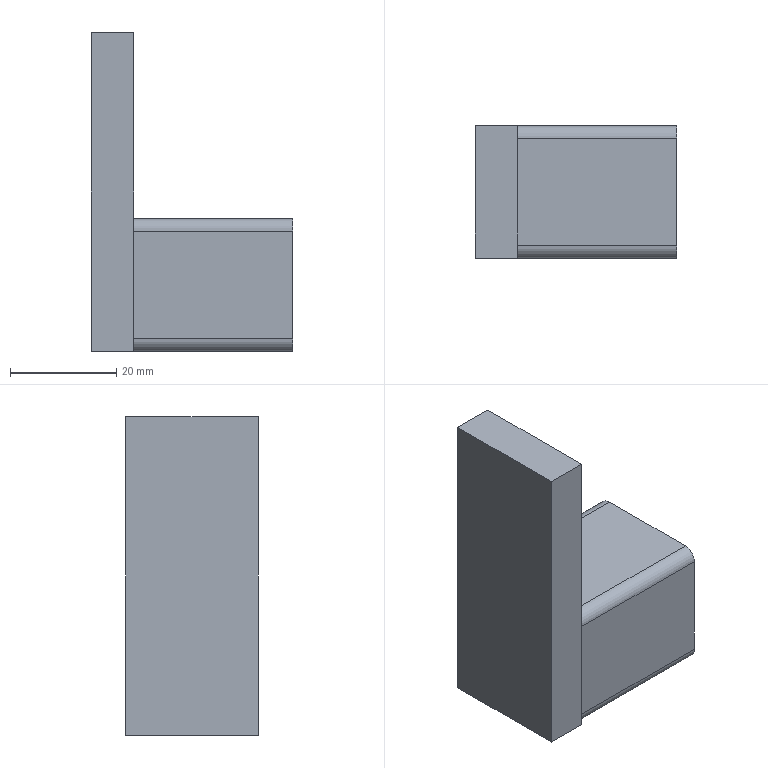Part | SolidWorks | features ICE 1, WeldMemberFeat 1, WeldmentFeature 1 | 2 solids | 24 faces | box 38 x 25 x 60 mm | volume 15316 mm3 | plane 16 | cylinder 8 | commonest cylinder face diameters 2.4 x4 4.8 x4
STEP:
#1=CARTESIAN_POINT('',(-15.,10.1,-12.5));
#2=VERTEX_POINT('',#1);
#3=CARTESIAN_POINT('',(-15.,12.5,-10.1));
#4=VERTEX_POINT('',#3);
#5=CARTESIAN_POINT('',(-15.,10.1,-10.1));
#6=DIRECTION('',(1.,0.,0.));
#7=DIRECTION('',(0.,0.,-1.));
#8=AXIS2_PLACEMENT_3D('',#5,#6,#7);
#9=CIRCLE('',#8,2.4);
#10=EDGE_CURVE('',#2,#4,#9,.T.);
#11=ORIENTED_EDGE('',*,*,#10,.T.);
#12=CARTESIAN_POINT('',(15.,12.5,-10.1));
#13=VERTEX_POINT('',#12);
#14=CARTESIAN_POINT('',(15.,12.5,-10.1));
#15=DIRECTION('',(-1.,0.,0.));
#16=VECTOR('',#15,1000.);
#17=LINE('',#14,#16);
#18=EDGE_CURVE('',#13,#4,#17,.T.);
#19=ORIENTED_EDGE('',*,*,#18,.F.);
#20=CARTESIAN_POINT('',(15.,10.1,-12.5));
#21=VERTEX_POINT('',#20);
#22=CARTESIAN_POINT('',(15.,10.1,-10.1));
#23=DIRECTION('',(1.,0.,0.));
#24=DIRECTION('',(0.,0.,-1.));
#25=AXIS2_PLACEMENT_3D('',#22,#23,#24);
#26=CIRCLE('',#25,2.4);
#27=EDGE_CURVE('',#21,#13,#26,.T.);
#28=ORIENTED_EDGE('',*,*,#27,.F.);
#29=CARTESIAN_POINT('',(15.,10.1,-12.5));
#30=DIRECTION('',(-1.,0.,0.));
#31=VECTOR('',#30,1000.);
#32=LINE('',#29,#31);
#33=EDGE_CURVE('',#21,#2,#32,.T.);
#34=ORIENTED_EDGE('',*,*,#33,.T.);
#35=EDGE_LOOP('',(#11,#19,#28,#34));
#36=FACE_OUTER_BOUND('',#35,.T.);
#37=CARTESIAN_POINT('',(15.,10.1,-10.1));
#38=DIRECTION('',(-1.,0.,0.));
#39=DIRECTION('',(0.,0.,1.));
#40=AXIS2_PLACEMENT_3D('',#37,#38,#39);
#41=CYLINDRICAL_SURFACE('',#40,2.4);
#42=ADVANCED_FACE('',(#36),#41,.T.);
#43=CARTESIAN_POINT('',(-15.,12.5,10.1));
#44=VERTEX_POINT('',#43);
#45=CARTESIAN_POINT('',(-15.,12.5,-10.1));
#46=DIRECTION('',(0.,0.,1.));
#47=VECTOR('',#46,1000.);
#48=LINE('',#45,#47);
#49=EDGE_CURVE('',#4,#44,#48,.T.);
#50=ORIENTED_EDGE('',*,*,#49,.T.);
#51=CARTESIAN_POINT('',(15.,12.5,10.1));
#52=VERTEX_POINT('',#51);
#53=CARTESIAN_POINT('',(15.,12.5,10.1));
#54=DIRECTION('',(-1.,0.,0.));
#55=VECTOR('',#54,1000.);
#56=LINE('',#53,#55);
#57=EDGE_CURVE('',#52,#44,#56,.T.);
#58=ORIENTED_EDGE('',*,*,#57,.F.);
#59=CARTESIAN_POINT('',(15.,12.5,-10.1));
#60=DIRECTION('',(0.,0.,1.));
#61=VECTOR('',#60,1000.);
#62=LINE('',#59,#61);
#63=EDGE_CURVE('',#13,#52,#62,.T.);
#64=ORIENTED_EDGE('',*,*,#63,.F.);
#65=ORIENTED_EDGE('',*,*,#18,.T.);
#66=EDGE_LOOP('',(#50,#58,#64,#65));
#67=FACE_OUTER_BOUND('',#66,.T.);
#68=CARTESIAN_POINT('',(15.,12.5,-10.1));
#69=DIRECTION('',(0.,-1.,0.));
#70=DIRECTION('',(0.,0.,-1.));
#71=AXIS2_PLACEMENT_3D('',#68,#69,#70);
#72=PLANE('',#71);
#73=ADVANCED_FACE('',(#67),#72,.F.);
#74=CARTESIAN_POINT('',(-15.,10.1,12.5));
#75=VERTEX_POINT('',#74);
#76=CARTESIAN_POINT('',(-15.,10.1,10.1));
#77=DIRECTION('',(1.,0.,0.));
#78=DIRECTION('',(0.,0.,-1.));
#79=AXIS2_PLACEMENT_3D('',#76,#77,#78);
#80=CIRCLE('',#79,2.4);
#81=EDGE_CURVE('',#44,#75,#80,.T.);
#82=ORIENTED_EDGE('',*,*,#81,.T.);
#83=CARTESIAN_POINT('',(15.,10.1,12.5));
#84=VERTEX_POINT('',#83);
#85=CARTESIAN_POINT('',(15.,10.1,12.5));
#86=DIRECTION('',(-1.,0.,0.));
#87=VECTOR('',#86,1000.);
#88=LINE('',#85,#87);
#89=EDGE_CURVE('',#84,#75,#88,.T.);
#90=ORIENTED_EDGE('',*,*,#89,.F.);
#91=CARTESIAN_POINT('',(15.,10.1,10.1));
#92=DIRECTION('',(1.,0.,0.));
#93=DIRECTION('',(0.,0.,-1.));
#94=AXIS2_PLACEMENT_3D('',#91,#92,#93);
#95=CIRCLE('',#94,2.4);
#96=EDGE_CURVE('',#52,#84,#95,.T.);
#97=ORIENTED_EDGE('',*,*,#96,.F.);
#98=ORIENTED_EDGE('',*,*,#57,.T.);
#99=EDGE_LOOP('',(#82,#90,#97,#98));
#100=FACE_OUTER_BOUND('',#99,.T.);
#101=CARTESIAN_POINT('',(15.,10.1,10.1));
#102=DIRECTION('',(-1.,0.,0.));
#103=DIRECTION('',(0.,0.,1.));
#104=AXIS2_PLACEMENT_3D('',#101,#102,#103);
#105=CYLINDRICAL_SURFACE('',#104,2.4);
#106=ADVANCED_FACE('',(#100),#105,.T.);
#107=CARTESIAN_POINT('',(-15.,-10.1,12.5));
#108=VERTEX_POINT('',#107);
#109=CARTESIAN_POINT('',(-15.,-10.1,12.5));
#110=DIRECTION('',(0.,-1.,0.));
#111=VECTOR('',#110,1000.);
#112=LINE('',#109,#111);
#113=EDGE_CURVE('',#75,#108,#112,.T.);
#114=ORIENTED_EDGE('',*,*,#113,.T.);
#115=CARTESIAN_POINT('',(15.,-10.1,12.5));
#116=VERTEX_POINT('',#115);
#117=CARTESIAN_POINT('',(15.,-10.1,12.5));
#118=DIRECTION('',(-1.,0.,0.));
#119=VECTOR('',#118,1000.);
#120=LINE('',#117,#119);
#121=EDGE_CURVE('',#116,#108,#120,.T.);
#122=ORIENTED_EDGE('',*,*,#121,.F.);
#123=CARTESIAN_POINT('',(15.,-10.1,12.5));
#124=DIRECTION('',(0.,-1.,0.));
#125=VECTOR('',#124,1000.);
#126=LINE('',#123,#125);
#127=EDGE_CURVE('',#84,#116,#126,.T.);
#128=ORIENTED_EDGE('',*,*,#127,.F.);
#129=ORIENTED_EDGE('',*,*,#89,.T.);
#130=EDGE_LOOP('',(#114,#122,#128,#129));
#131=FACE_OUTER_BOUND('',#130,.T.);
#132=CARTESIAN_POINT('',(15.,-10.1,12.5));
#133=DIRECTION('',(0.,0.,-1.));
#134=DIRECTION('',(-1.,0.,0.));
#135=AXIS2_PLACEMENT_3D('',#132,#133,#134);
#136=PLANE('',#135);
#137=ADVANCED_FACE('',(#131),#136,.F.);
#138=CARTESIAN_POINT('',(-15.,-12.5,10.1));
#139=VERTEX_POINT('',#138);
#140=CARTESIAN_POINT('',(-15.,-10.1,10.1));
#141=DIRECTION('',(1.,0.,0.));
#142=DIRECTION('',(0.,0.,-1.));
#143=AXIS2_PLACEMENT_3D('',#140,#141,#142);
#144=CIRCLE('',#143,2.4);
#145=EDGE_CURVE('',#108,#139,#144,.T.);
#146=ORIENTED_EDGE('',*,*,#145,.T.);
#147=CARTESIAN_POINT('',(15.,-12.5,10.1));
#148=VERTEX_POINT('',#147);
#149=CARTESIAN_POINT('',(15.,-12.5,10.1));
#150=DIRECTION('',(-1.,0.,0.));
#151=VECTOR('',#150,1000.);
#152=LINE('',#149,#151);
#153=EDGE_CURVE('',#148,#139,#152,.T.);
#154=ORIENTED_EDGE('',*,*,#153,.F.);
#155=CARTESIAN_POINT('',(15.,-10.1,10.1));
#156=DIRECTION('',(1.,0.,0.));
#157=DIRECTION('',(0.,0.,-1.));
#158=AXIS2_PLACEMENT_3D('',#155,#156,#157);
#159=CIRCLE('',#158,2.4);
#160=EDGE_CURVE('',#116,#148,#159,.T.);
#161=ORIENTED_EDGE('',*,*,#160,.F.);
#162=ORIENTED_EDGE('',*,*,#121,.T.);
#163=EDGE_LOOP('',(#146,#154,#161,#162));
#164=FACE_OUTER_BOUND('',#163,.T.);
#165=CARTESIAN_POINT('',(15.,-10.1,10.1));
#166=DIRECTION('',(-1.,0.,0.));
#167=DIRECTION('',(0.,0.,1.));
#168=AXIS2_PLACEMENT_3D('',#165,#166,#167);
#169=CYLINDRICAL_SURFACE('',#168,2.4);
#170=ADVANCED_FACE('',(#164),#169,.T.);
#171=CARTESIAN_POINT('',(-15.,-12.5,-10.1));
#172=VERTEX_POINT('',#171);
#173=CARTESIAN_POINT('',(-15.,-12.5,10.1));
#174=DIRECTION('',(0.,0.,-1.));
#175=VECTOR('',#174,1000.);
#176=LINE('',#173,#175);
#177=EDGE_CURVE('',#139,#172,#176,.T.);
#178=ORIENTED_EDGE('',*,*,#177,.T.);
#179=CARTESIAN_POINT('',(15.,-12.5,-10.1));
#180=VERTEX_POINT('',#179);
#181=CARTESIAN_POINT('',(15.,-12.5,-10.1));
#182=DIRECTION('',(-1.,0.,0.));
#183=VECTOR('',#182,1000.);
#184=LINE('',#181,#183);
#185=EDGE_CURVE('',#180,#172,#184,.T.);
#186=ORIENTED_EDGE('',*,*,#185,.F.);
#187=CARTESIAN_POINT('',(15.,-12.5,10.1));
#188=DIRECTION('',(0.,0.,-1.));
#189=VECTOR('',#188,1000.);
#190=LINE('',#187,#189);
#191=EDGE_CURVE('',#148,#180,#190,.T.);
#192=ORIENTED_EDGE('',*,*,#191,.F.);
#193=ORIENTED_EDGE('',*,*,#153,.T.);
#194=EDGE_LOOP('',(#178,#186,#192,#193));
#195=FACE_OUTER_BOUND('',#194,.T.);
#196=CARTESIAN_POINT('',(15.,-12.5,10.1));
#197=DIRECTION('',(0.,1.,0.));
#198=DIRECTION('',(0.,0.,1.));
#199=AXIS2_PLACEMENT_3D('',#196,#197,#198);
#200=PLANE('',#199);
#201=ADVANCED_FACE('',(#195),#200,.F.);
#202=CARTESIAN_POINT('',(-15.,-10.1,-12.5));
#203=VERTEX_POINT('',#202);
#204=CARTESIAN_POINT('',(-15.,-10.1,-10.1));
#205=DIRECTION('',(1.,0.,0.));
#206=DIRECTION('',(0.,0.,-1.));
#207=AXIS2_PLACEMENT_3D('',#204,#205,#206);
#208=CIRCLE('',#207,2.4);
#209=EDGE_CURVE('',#172,#203,#208,.T.);
#210=ORIENTED_EDGE('',*,*,#209,.T.);
#211=CARTESIAN_POINT('',(15.,-10.1,-12.5));
#212=VERTEX_POINT('',#211);
#213=CARTESIAN_POINT('',(15.,-10.1,-12.5));
#214=DIRECTION('',(-1.,0.,0.));
#215=VECTOR('',#214,1000.);
#216=LINE('',#213,#215);
#217=EDGE_CURVE('',#212,#203,#216,.T.);
#218=ORIENTED_EDGE('',*,*,#217,.F.);
#219=CARTESIAN_POINT('',(15.,-10.1,-10.1));
#220=DIRECTION('',(1.,0.,0.));
#221=DIRECTION('',(0.,0.,-1.));
#222=AXIS2_PLACEMENT_3D('',#219,#220,#221);
#223=CIRCLE('',#222,2.4);
#224=EDGE_CURVE('',#180,#212,#223,.T.);
#225=ORIENTED_EDGE('',*,*,#224,.F.);
#226=ORIENTED_EDGE('',*,*,#185,.T.);
#227=EDGE_LOOP('',(#210,#218,#225,#226));
#228=FACE_OUTER_BOUND('',#227,.T.);
#229=CARTESIAN_POINT('',(15.,-10.1,-10.1));
#230=DIRECTION('',(-1.,0.,0.));
#231=DIRECTION('',(0.,0.,1.));
#232=AXIS2_PLACEMENT_3D('',#229,#230,#231);
#233=CYLINDRICAL_SURFACE('',#232,2.4);
#234=ADVANCED_FACE('',(#228),#233,.T.);
#235=CARTESIAN_POINT('',(-15.,11.3,10.1));
#236=VERTEX_POINT('',#235);
#237=CARTESIAN_POINT('',(-15.,10.1,11.3));
#238=VERTEX_POINT('',#237);
#239=CARTESIAN_POINT('',(-15.,10.1,10.1));
#240=DIRECTION('',(1.,0.,0.));
#241=DIRECTION('',(0.,0.,-1.));
#242=AXIS2_PLACEMENT_3D('',#239,#240,#241);
#243=CIRCLE('',#242,1.2);
#244=EDGE_CURVE('',#236,#238,#243,.T.);
#245=ORIENTED_EDGE('',*,*,#244,.F.);
#246=CARTESIAN_POINT('',(15.,11.3,10.1));
#247=VERTEX_POINT('',#246);
#248=CARTESIAN_POINT('',(15.,11.3,10.1));
#249=DIRECTION('',(-1.,0.,0.));
#250=VECTOR('',#249,1000.);
#251=LINE('',#248,#250);
#252=EDGE_CURVE('',#247,#236,#251,.T.);
#253=ORIENTED_EDGE('',*,*,#252,.F.);
#254=CARTESIAN_POINT('',(15.,10.1,11.3));
#255=VERTEX_POINT('',#254);
#256=CARTESIAN_POINT('',(15.,10.1,10.1));
#257=DIRECTION('',(1.,0.,0.));
#258=DIRECTION('',(0.,0.,-1.));
#259=AXIS2_PLACEMENT_3D('',#256,#257,#258);
#260=CIRCLE('',#259,1.2);
#261=EDGE_CURVE('',#247,#255,#260,.T.);
#262=ORIENTED_EDGE('',*,*,#261,.T.);
#263=CARTESIAN_POINT('',(15.,10.1,11.3));
#264=DIRECTION('',(-1.,0.,0.));
#265=VECTOR('',#264,1000.);
#266=LINE('',#263,#265);
#267=EDGE_CURVE('',#255,#238,#266,.T.);
#268=ORIENTED_EDGE('',*,*,#267,.T.);
#269=EDGE_LOOP('',(#245,#253,#262,#268));
#270=FACE_OUTER_BOUND('',#269,.T.);
#271=CARTESIAN_POINT('',(15.,10.1,10.1));
#272=DIRECTION('',(-1.,0.,0.));
#273=DIRECTION('',(0.,0.,1.));
#274=AXIS2_PLACEMENT_3D('',#271,#272,#273);
#275=CYLINDRICAL_SURFACE('',#274,1.2);
#276=ADVANCED_FACE('',(#270),#275,.F.);
#277=CARTESIAN_POINT('',(-15.,11.3,-10.1));
#278=VERTEX_POINT('',#277);
#279=CARTESIAN_POINT('',(-15.,11.3,-10.1));
#280=DIRECTION('',(0.,0.,1.));
#281=VECTOR('',#280,1000.);
#282=LINE('',#279,#281);
#283=EDGE_CURVE('',#278,#236,#282,.T.);
#284=ORIENTED_EDGE('',*,*,#283,.F.);
#285=CARTESIAN_POINT('',(15.,11.3,-10.1));
#286=VERTEX_POINT('',#285);
#287=CARTESIAN_POINT('',(15.,11.3,-10.1));
#288=DIRECTION('',(-1.,0.,0.));
#289=VECTOR('',#288,1000.);
#290=LINE('',#287,#289);
#291=EDGE_CURVE('',#286,#278,#290,.T.);
#292=ORIENTED_EDGE('',*,*,#291,.F.);
#293=CARTESIAN_POINT('',(15.,11.3,-10.1));
#294=DIRECTION('',(0.,0.,1.));
#295=VECTOR('',#294,1000.);
#296=LINE('',#293,#295);
#297=EDGE_CURVE('',#286,#247,#296,.T.);
#298=ORIENTED_EDGE('',*,*,#297,.T.);
#299=ORIENTED_EDGE('',*,*,#252,.T.);
#300=EDGE_LOOP('',(#284,#292,#298,#299));
#301=FACE_OUTER_BOUND('',#300,.T.);
#302=CARTESIAN_POINT('',(15.,11.3,-10.1));
#303=DIRECTION('',(0.,-1.,0.));
#304=DIRECTION('',(0.,0.,-1.));
#305=AXIS2_PLACEMENT_3D('',#302,#303,#304);
#306=PLANE('',#305);
#307=ADVANCED_FACE('',(#301),#306,.T.);
#308=CARTESIAN_POINT('',(-15.,10.1,-11.3));
#309=VERTEX_POINT('',#308);
#310=CARTESIAN_POINT('',(-15.,10.1,-10.1));
#311=DIRECTION('',(1.,0.,0.));
#312=DIRECTION('',(0.,0.,-1.));
#313=AXIS2_PLACEMENT_3D('',#310,#311,#312);
#314=CIRCLE('',#313,1.2);
#315=EDGE_CURVE('',#309,#278,#314,.T.);
#316=ORIENTED_EDGE('',*,*,#315,.F.);
#317=CARTESIAN_POINT('',(15.,10.1,-11.3));
#318=VERTEX_POINT('',#317);
#319=CARTESIAN_POINT('',(15.,10.1,-11.3));
#320=DIRECTION('',(-1.,0.,0.));
#321=VECTOR('',#320,1000.);
#322=LINE('',#319,#321);
#323=EDGE_CURVE('',#318,#309,#322,.T.);
#324=ORIENTED_EDGE('',*,*,#323,.F.);
#325=CARTESIAN_POINT('',(15.,10.1,-10.1));
#326=DIRECTION('',(1.,0.,0.));
#327=DIRECTION('',(0.,0.,-1.));
#328=AXIS2_PLACEMENT_3D('',#325,#326,#327);
#329=CIRCLE('',#328,1.2);
#330=EDGE_CURVE('',#318,#286,#329,.T.);
#331=ORIENTED_EDGE('',*,*,#330,.T.);
#332=ORIENTED_EDGE('',*,*,#291,.T.);
#333=EDGE_LOOP('',(#316,#324,#331,#332));
#334=FACE_OUTER_BOUND('',#333,.T.);
#335=CARTESIAN_POINT('',(15.,10.1,-10.1));
#336=DIRECTION('',(-1.,0.,0.));
#337=DIRECTION('',(0.,0.,1.));
#338=AXIS2_PLACEMENT_3D('',#335,#336,#337);
#339=CYLINDRICAL_SURFACE('',#338,1.2);
#340=ADVANCED_FACE('',(#334),#339,.F.);
#341=CARTESIAN_POINT('',(-15.,-10.1,-11.3));
#342=VERTEX_POINT('',#341);
#343=CARTESIAN_POINT('',(-15.,10.1,-11.3));
#344=DIRECTION('',(0.,1.,0.));
#345=VECTOR('',#344,1000.);
#346=LINE('',#343,#345);
#347=EDGE_CURVE('',#342,#309,#346,.T.);
#348=ORIENTED_EDGE('',*,*,#347,.F.);
#349=CARTESIAN_POINT('',(15.,-10.1,-11.3));
#350=VERTEX_POINT('',#349);
#351=CARTESIAN_POINT('',(15.,-10.1,-11.3));
#352=DIRECTION('',(-1.,0.,0.));
#353=VECTOR('',#352,1000.);
#354=LINE('',#351,#353);
#355=EDGE_CURVE('',#350,#342,#354,.T.);
#356=ORIENTED_EDGE('',*,*,#355,.F.);
#357=CARTESIAN_POINT('',(15.,10.1,-11.3));
#358=DIRECTION('',(0.,1.,0.));
#359=VECTOR('',#358,1000.);
#360=LINE('',#357,#359);
#361=EDGE_CURVE('',#350,#318,#360,.T.);
#362=ORIENTED_EDGE('',*,*,#361,.T.);
#363=ORIENTED_EDGE('',*,*,#323,.T.);
#364=EDGE_LOOP('',(#348,#356,#362,#363));
#365=FACE_OUTER_BOUND('',#364,.T.);
#366=CARTESIAN_POINT('',(15.,10.1,-11.3));
#367=DIRECTION('',(0.,0.,1.));
#368=DIRECTION('',(1.,0.,0.));
#369=AXIS2_PLACEMENT_3D('',#366,#367,#368);
#370=PLANE('',#369);
#371=ADVANCED_FACE('',(#365),#370,.T.);
#372=CARTESIAN_POINT('',(-15.,-11.3,-10.1));
#373=VERTEX_POINT('',#372);
#374=CARTESIAN_POINT('',(-15.,-10.1,-10.1));
#375=DIRECTION('',(1.,0.,0.));
#376=DIRECTION('',(0.,0.,-1.));
#377=AXIS2_PLACEMENT_3D('',#374,#375,#376);
#378=CIRCLE('',#377,1.2);
#379=EDGE_CURVE('',#373,#342,#378,.T.);
#380=ORIENTED_EDGE('',*,*,#379,.F.);
#381=CARTESIAN_POINT('',(15.,-11.3,-10.1));
#382=VERTEX_POINT('',#381);
#383=CARTESIAN_POINT('',(15.,-11.3,-10.1));
#384=DIRECTION('',(-1.,0.,0.));
#385=VECTOR('',#384,1000.);
#386=LINE('',#383,#385);
#387=EDGE_CURVE('',#382,#373,#386,.T.);
#388=ORIENTED_EDGE('',*,*,#387,.F.);
#389=CARTESIAN_POINT('',(15.,-10.1,-10.1));
#390=DIRECTION('',(1.,0.,0.));
#391=DIRECTION('',(0.,0.,-1.));
#392=AXIS2_PLACEMENT_3D('',#389,#390,#391);
#393=CIRCLE('',#392,1.2);
#394=EDGE_CURVE('',#382,#350,#393,.T.);
#395=ORIENTED_EDGE('',*,*,#394,.T.);
#396=ORIENTED_EDGE('',*,*,#355,.T.);
#397=EDGE_LOOP('',(#380,#388,#395,#396));
#398=FACE_OUTER_BOUND('',#397,.T.);
#399=CARTESIAN_POINT('',(15.,-10.1,-10.1));
#400=DIRECTION('',(-1.,0.,0.));
#401=DIRECTION('',(0.,0.,1.));
#402=AXIS2_PLACEMENT_3D('',#399,#400,#401);
#403=CYLINDRICAL_SURFACE('',#402,1.2);
#404=ADVANCED_FACE('',(#398),#403,.F.);
#405=CARTESIAN_POINT('',(-15.,-11.3,10.1));
#406=VERTEX_POINT('',#405);
#407=CARTESIAN_POINT('',(-15.,-11.3,10.1));
#408=DIRECTION('',(0.,0.,-1.));
#409=VECTOR('',#408,1000.);
#410=LINE('',#407,#409);
#411=EDGE_CURVE('',#406,#373,#410,.T.);
#412=ORIENTED_EDGE('',*,*,#411,.F.);
#413=CARTESIAN_POINT('',(15.,-11.3,10.1));
#414=VERTEX_POINT('',#413);
#415=CARTESIAN_POINT('',(15.,-11.3,10.1));
#416=DIRECTION('',(-1.,0.,0.));
#417=VECTOR('',#416,1000.);
#418=LINE('',#415,#417);
#419=EDGE_CURVE('',#414,#406,#418,.T.);
#420=ORIENTED_EDGE('',*,*,#419,.F.);
#421=CARTESIAN_POINT('',(15.,-11.3,10.1));
#422=DIRECTION('',(0.,0.,-1.));
#423=VECTOR('',#422,1000.);
#424=LINE('',#421,#423);
#425=EDGE_CURVE('',#414,#382,#424,.T.);
#426=ORIENTED_EDGE('',*,*,#425,.T.);
#427=ORIENTED_EDGE('',*,*,#387,.T.);
#428=EDGE_LOOP('',(#412,#420,#426,#427));
#429=FACE_OUTER_BOUND('',#428,.T.);
#430=CARTESIAN_POINT('',(15.,-11.3,10.1));
#431=DIRECTION('',(0.,1.,0.));
#432=DIRECTION('',(0.,0.,1.));
#433=AXIS2_PLACEMENT_3D('',#430,#431,#432);
#434=PLANE('',#433);
#435=ADVANCED_FACE('',(#429),#434,.T.);
#436=CARTESIAN_POINT('',(-15.,-10.1,11.3));
#437=VERTEX_POINT('',#436);
#438=CARTESIAN_POINT('',(-15.,-10.1,10.1));
#439=DIRECTION('',(1.,0.,0.));
#440=DIRECTION('',(0.,0.,-1.));
#441=AXIS2_PLACEMENT_3D('',#438,#439,#440);
#442=CIRCLE('',#441,1.2);
#443=EDGE_CURVE('',#437,#406,#442,.T.);
#444=ORIENTED_EDGE('',*,*,#443,.F.);
#445=CARTESIAN_POINT('',(15.,-10.1,11.3));
#446=VERTEX_POINT('',#445);
#447=CARTESIAN_POINT('',(15.,-10.1,11.3));
#448=DIRECTION('',(-1.,0.,0.));
#449=VECTOR('',#448,1000.);
#450=LINE('',#447,#449);
#451=EDGE_CURVE('',#446,#437,#450,.T.);
#452=ORIENTED_EDGE('',*,*,#451,.F.);
#453=CARTESIAN_POINT('',(15.,-10.1,10.1));
#454=DIRECTION('',(1.,0.,0.));
#455=DIRECTION('',(0.,0.,-1.));
#456=AXIS2_PLACEMENT_3D('',#453,#454,#455);
#457=CIRCLE('',#456,1.2);
#458=EDGE_CURVE('',#446,#414,#457,.T.);
#459=ORIENTED_EDGE('',*,*,#458,.T.);
#460=ORIENTED_EDGE('',*,*,#419,.T.);
#461=EDGE_LOOP('',(#444,#452,#459,#460));
#462=FACE_OUTER_BOUND('',#461,.T.);
#463=CARTESIAN_POINT('',(15.,-10.1,10.1));
#464=DIRECTION('',(-1.,0.,0.));
#465=DIRECTION('',(0.,0.,1.));
#466=AXIS2_PLACEMENT_3D('',#463,#464,#465);
#467=CYLINDRICAL_SURFACE('',#466,1.2);
#468=ADVANCED_FACE('',(#462),#467,.F.);
#469=CARTESIAN_POINT('',(-15.,-10.1,11.3));
#470=DIRECTION('',(0.,-1.,0.));
#471=VECTOR('',#470,1000.);
#472=LINE('',#469,#471);
#473=EDGE_CURVE('',#238,#437,#472,.T.);
#474=ORIENTED_EDGE('',*,*,#473,.F.);
#475=ORIENTED_EDGE('',*,*,#267,.F.);
#476=CARTESIAN_POINT('',(15.,-10.1,11.3));
#477=DIRECTION('',(0.,-1.,0.));
#478=VECTOR('',#477,1000.);
#479=LINE('',#476,#478);
#480=EDGE_CURVE('',#255,#446,#479,.T.);
#481=ORIENTED_EDGE('',*,*,#480,.T.);
#482=ORIENTED_EDGE('',*,*,#451,.T.);
#483=EDGE_LOOP('',(#474,#475,#481,#482));
#484=FACE_OUTER_BOUND('',#483,.T.);
#485=CARTESIAN_POINT('',(15.,-10.1,11.3));
#486=DIRECTION('',(0.,0.,-1.));
#487=DIRECTION('',(-1.,0.,0.));
#488=AXIS2_PLACEMENT_3D('',#485,#486,#487);
#489=PLANE('',#488);
#490=ADVANCED_FACE('',(#484),#489,.T.);
#491=CARTESIAN_POINT('',(-15.,10.1,-12.5));
#492=DIRECTION('',(0.,1.,0.));
#493=VECTOR('',#492,1000.);
#494=LINE('',#491,#493);
#495=EDGE_CURVE('',#203,#2,#494,.T.);
#496=ORIENTED_EDGE('',*,*,#495,.T.);
#497=ORIENTED_EDGE('',*,*,#33,.F.);
#498=CARTESIAN_POINT('',(15.,10.1,-12.5));
#499=DIRECTION('',(0.,1.,0.));
#500=VECTOR('',#499,1000.);
#501=LINE('',#498,#500);
#502=EDGE_CURVE('',#212,#21,#501,.T.);
#503=ORIENTED_EDGE('',*,*,#502,.F.);
#504=ORIENTED_EDGE('',*,*,#217,.T.);
#505=EDGE_LOOP('',(#496,#497,#503,#504));
#506=FACE_OUTER_BOUND('',#505,.T.);
#507=CARTESIAN_POINT('',(15.,10.1,-12.5));
#508=DIRECTION('',(0.,0.,1.));
#509=DIRECTION('',(1.,0.,0.));
#510=AXIS2_PLACEMENT_3D('',#507,#508,#509);
#511=PLANE('',#510);
#512=ADVANCED_FACE('',(#506),#511,.F.);
#513=ORIENTED_EDGE('',*,*,#261,.F.);
#514=ORIENTED_EDGE('',*,*,#297,.F.);
#515=ORIENTED_EDGE('',*,*,#330,.F.);
#516=ORIENTED_EDGE('',*,*,#361,.F.);
#517=ORIENTED_EDGE('',*,*,#394,.F.);
#518=ORIENTED_EDGE('',*,*,#425,.F.);
#519=ORIENTED_EDGE('',*,*,#458,.F.);
#520=ORIENTED_EDGE('',*,*,#480,.F.);
#521=EDGE_LOOP('',(#513,#514,#515,#516,#517,#518,#519,#520));
#522=FACE_BOUND('',#521,.T.);
#523=ORIENTED_EDGE('',*,*,#27,.T.);
#524=ORIENTED_EDGE('',*,*,#63,.T.);
#525=ORIENTED_EDGE('',*,*,#96,.T.);
#526=ORIENTED_EDGE('',*,*,#127,.T.);
#527=ORIENTED_EDGE('',*,*,#160,.T.);
#528=ORIENTED_EDGE('',*,*,#191,.T.);
#529=ORIENTED_EDGE('',*,*,#224,.T.);
#530=ORIENTED_EDGE('',*,*,#502,.T.);
#531=EDGE_LOOP('',(#523,#524,#525,#526,#527,#528,#529,#530));
#532=FACE_OUTER_BOUND('',#531,.T.);
#533=CARTESIAN_POINT('',(15.,10.1,-10.1));
#534=DIRECTION('',(1.,0.,0.));
#535=DIRECTION('',(0.,0.,-1.));
#536=AXIS2_PLACEMENT_3D('',#533,#534,#535);
#537=PLANE('',#536);
#538=ADVANCED_FACE('',(#522,#532),#537,.T.);
#539=ORIENTED_EDGE('',*,*,#244,.T.);
#540=ORIENTED_EDGE('',*,*,#473,.T.);
#541=ORIENTED_EDGE('',*,*,#443,.T.);
#542=ORIENTED_EDGE('',*,*,#411,.T.);
#543=ORIENTED_EDGE('',*,*,#379,.T.);
#544=ORIENTED_EDGE('',*,*,#347,.T.);
#545=ORIENTED_EDGE('',*,*,#315,.T.);
#546=ORIENTED_EDGE('',*,*,#283,.T.);
#547=EDGE_LOOP('',(#539,#540,#541,#542,#543,#544,#545,#546));
#548=FACE_BOUND('',#547,.T.);
#549=ORIENTED_EDGE('',*,*,#10,.F.);
#550=ORIENTED_EDGE('',*,*,#495,.F.);
#551=ORIENTED_EDGE('',*,*,#209,.F.);
#552=ORIENTED_EDGE('',*,*,#177,.F.);
#553=ORIENTED_EDGE('',*,*,#145,.F.);
#554=ORIENTED_EDGE('',*,*,#113,.F.);
#555=ORIENTED_EDGE('',*,*,#81,.F.);
#556=ORIENTED_EDGE('',*,*,#49,.F.);
#557=EDGE_LOOP('',(#549,#550,#551,#552,#553,#554,#555,#556));
#558=FACE_OUTER_BOUND('',#557,.T.);
#559=CARTESIAN_POINT('',(-15.,10.1,-10.1));
#560=DIRECTION('',(1.,0.,0.));
#561=DIRECTION('',(0.,0.,-1.));
#562=AXIS2_PLACEMENT_3D('',#559,#560,#561);
#563=PLANE('',#562);
#564=ADVANCED_FACE('',(#548,#558),#563,.F.);
#565=CLOSED_SHELL('',(#42,#73,#106,#137,#170,#201,#234,#276,#307,#340,#371,#404,#435,#468,#490,#512,#538,#564));
#566=MANIFOLD_SOLID_BREP('',#565);
#567=CARTESIAN_POINT('',(-15.,12.5,-12.5));
#568=VERTEX_POINT('',#567);
#569=CARTESIAN_POINT('',(-15.,-12.5,-12.5));
#570=VERTEX_POINT('',#569);
#571=CARTESIAN_POINT('',(-15.,12.5,-12.5));
#572=DIRECTION('',(0.,-1.,0.));
#573=VECTOR('',#572,1000.);
#574=LINE('',#571,#573);
#575=EDGE_CURVE('',#568,#570,#574,.T.);
#576=ORIENTED_EDGE('',*,*,#575,.T.);
#577=CARTESIAN_POINT('',(-23.,-12.5,-12.5));
#578=VERTEX_POINT('',#577);
#579=CARTESIAN_POINT('',(-23.,-12.5,-12.5));
#580=DIRECTION('',(1.,0.,0.));
#581=VECTOR('',#580,1000.);
#582=LINE('',#579,#581);
#583=EDGE_CURVE('',#578,#570,#582,.T.);
#584=ORIENTED_EDGE('',*,*,#583,.F.);
#585=CARTESIAN_POINT('',(-23.,12.5,-12.5));
#586=VERTEX_POINT('',#585);
#587=CARTESIAN_POINT('',(-23.,12.5,-12.5));
#588=DIRECTION('',(0.,-1.,0.));
#589=VECTOR('',#588,1000.);
#590=LINE('',#587,#589);
#591=EDGE_CURVE('',#586,#578,#590,.T.);
#592=ORIENTED_EDGE('',*,*,#591,.F.);
#593=CARTESIAN_POINT('',(-23.,12.5,-12.5));
#594=DIRECTION('',(1.,0.,0.));
#595=VECTOR('',#594,1000.);
#596=LINE('',#593,#595);
#597=EDGE_CURVE('',#586,#568,#596,.T.);
#598=ORIENTED_EDGE('',*,*,#597,.T.);
#599=EDGE_LOOP('',(#576,#584,#592,#598));
#600=FACE_OUTER_BOUND('',#599,.T.);
#601=CARTESIAN_POINT('',(-23.,12.5,-12.5));
#602=DIRECTION('',(0.,0.,1.));
#603=DIRECTION('',(0.,-1.,0.));
#604=AXIS2_PLACEMENT_3D('',#601,#602,#603);
#605=PLANE('',#604);
#606=ADVANCED_FACE('',(#600),#605,.F.);
#607=CARTESIAN_POINT('',(-15.,-12.5,47.5));
#608=VERTEX_POINT('',#607);
#609=CARTESIAN_POINT('',(-15.,-12.5,-12.5));
#610=DIRECTION('',(0.,0.,1.));
#611=VECTOR('',#610,1000.);
#612=LINE('',#609,#611);
#613=EDGE_CURVE('',#570,#608,#612,.T.);
#614=ORIENTED_EDGE('',*,*,#613,.T.);
#615=CARTESIAN_POINT('',(-23.,-12.5,47.5));
#616=VERTEX_POINT('',#615);
#617=CARTESIAN_POINT('',(-23.,-12.5,47.5));
#618=DIRECTION('',(1.,0.,0.));
#619=VECTOR('',#618,1000.);
#620=LINE('',#617,#619);
#621=EDGE_CURVE('',#616,#608,#620,.T.);
#622=ORIENTED_EDGE('',*,*,#621,.F.);
#623=CARTESIAN_POINT('',(-23.,-12.5,-12.5));
#624=DIRECTION('',(0.,0.,1.));
#625=VECTOR('',#624,1000.);
#626=LINE('',#623,#625);
#627=EDGE_CURVE('',#578,#616,#626,.T.);
#628=ORIENTED_EDGE('',*,*,#627,.F.);
#629=ORIENTED_EDGE('',*,*,#583,.T.);
#630=EDGE_LOOP('',(#614,#622,#628,#629));
#631=FACE_OUTER_BOUND('',#630,.T.);
#632=CARTESIAN_POINT('',(-23.,-12.5,-12.5));
#633=DIRECTION('',(0.,1.,0.));
#634=DIRECTION('',(0.,0.,1.));
#635=AXIS2_PLACEMENT_3D('',#632,#633,#634);
#636=PLANE('',#635);
#637=ADVANCED_FACE('',(#631),#636,.F.);
#638=CARTESIAN_POINT('',(-15.,12.5,47.5));
#639=VERTEX_POINT('',#638);
#640=CARTESIAN_POINT('',(-15.,12.5,47.5));
#641=DIRECTION('',(0.,1.,0.));
#642=VECTOR('',#641,1000.);
#643=LINE('',#640,#642);
#644=EDGE_CURVE('',#608,#639,#643,.T.);
#645=ORIENTED_EDGE('',*,*,#644,.T.);
#646=CARTESIAN_POINT('',(-23.,12.5,47.5));
#647=VERTEX_POINT('',#646);
#648=CARTESIAN_POINT('',(-23.,12.5,47.5));
#649=DIRECTION('',(1.,0.,0.));
#650=VECTOR('',#649,1000.);
#651=LINE('',#648,#650);
#652=EDGE_CURVE('',#647,#639,#651,.T.);
#653=ORIENTED_EDGE('',*,*,#652,.F.);
#654=CARTESIAN_POINT('',(-23.,12.5,47.5));
#655=DIRECTION('',(0.,1.,0.));
#656=VECTOR('',#655,1000.);
#657=LINE('',#654,#656);
#658=EDGE_CURVE('',#616,#647,#657,.T.);
#659=ORIENTED_EDGE('',*,*,#658,.F.);
#660=ORIENTED_EDGE('',*,*,#621,.T.);
#661=EDGE_LOOP('',(#645,#653,#659,#660));
#662=FACE_OUTER_BOUND('',#661,.T.);
#663=CARTESIAN_POINT('',(-23.,12.5,47.5));
#664=DIRECTION('',(0.,0.,-1.));
#665=DIRECTION('',(-1.,0.,0.));
#666=AXIS2_PLACEMENT_3D('',#663,#664,#665);
#667=PLANE('',#666);
#668=ADVANCED_FACE('',(#662),#667,.F.);
#669=CARTESIAN_POINT('',(-15.,12.5,-12.5));
#670=DIRECTION('',(0.,0.,-1.));
#671=VECTOR('',#670,1000.);
#672=LINE('',#669,#671);
#673=EDGE_CURVE('',#639,#568,#672,.T.);
#674=ORIENTED_EDGE('',*,*,#673,.T.);
#675=ORIENTED_EDGE('',*,*,#597,.F.);
#676=CARTESIAN_POINT('',(-23.,12.5,-12.5));
#677=DIRECTION('',(0.,0.,-1.));
#678=VECTOR('',#677,1000.);
#679=LINE('',#676,#678);
#680=EDGE_CURVE('',#647,#586,#679,.T.);
#681=ORIENTED_EDGE('',*,*,#680,.F.);
#682=ORIENTED_EDGE('',*,*,#652,.T.);
#683=EDGE_LOOP('',(#674,#675,#681,#682));
#684=FACE_OUTER_BOUND('',#683,.T.);
#685=CARTESIAN_POINT('',(-23.,12.5,-12.5));
#686=DIRECTION('',(0.,-1.,0.));
#687=DIRECTION('',(0.,0.,-1.));
#688=AXIS2_PLACEMENT_3D('',#685,#686,#687);
#689=PLANE('',#688);
#690=ADVANCED_FACE('',(#684),#689,.F.);
#691=ORIENTED_EDGE('',*,*,#591,.T.);
#692=ORIENTED_EDGE('',*,*,#627,.T.);
#693=ORIENTED_EDGE('',*,*,#658,.T.);
#694=ORIENTED_EDGE('',*,*,#680,.T.);
#695=EDGE_LOOP('',(#691,#692,#693,#694));
#696=FACE_OUTER_BOUND('',#695,.T.);
#697=CARTESIAN_POINT('',(-23.,0.,0.));
#698=DIRECTION('',(-1.,0.,0.));
#699=DIRECTION('',(0.,0.,1.));
#700=AXIS2_PLACEMENT_3D('',#697,#698,#699);
#701=PLANE('',#700);
#702=ADVANCED_FACE('',(#696),#701,.T.);
#703=ORIENTED_EDGE('',*,*,#575,.F.);
#704=ORIENTED_EDGE('',*,*,#673,.F.);
#705=ORIENTED_EDGE('',*,*,#644,.F.);
#706=ORIENTED_EDGE('',*,*,#613,.F.);
#707=EDGE_LOOP('',(#703,#704,#705,#706));
#708=FACE_OUTER_BOUND('',#707,.T.);
#709=CARTESIAN_POINT('',(-15.,0.,0.));
#710=DIRECTION('',(-1.,0.,0.));
#711=DIRECTION('',(0.,0.,1.));
#712=AXIS2_PLACEMENT_3D('',#709,#710,#711);
#713=PLANE('',#712);
#714=ADVANCED_FACE('',(#708),#713,.F.);
#715=CLOSED_SHELL('',(#606,#637,#668,#690,#702,#714));
#716=MANIFOLD_SOLID_BREP('',#715);
#717=CARTESIAN_POINT('',(0.,0.,0.));
#718=DIRECTION('',(0.,0.,1.));
#719=DIRECTION('',(1.,0.,0.));
#720=AXIS2_PLACEMENT_3D('',#717,#718,#719);
#721=(LENGTH_UNIT()NAMED_UNIT(*)SI_UNIT(.MILLI.,.METRE.));
#722=UNCERTAINTY_MEASURE_WITH_UNIT(LENGTH_MEASURE(0.00001),#721,'','');
#723=(NAMED_UNIT(*)PLANE_ANGLE_UNIT()SI_UNIT($,.RADIAN.));
#724=(NAMED_UNIT(*)SI_UNIT($,.STERADIAN.)SOLID_ANGLE_UNIT());
#725=(GEOMETRIC_REPRESENTATION_CONTEXT(3)GLOBAL_UNCERTAINTY_ASSIGNED_CONTEXT((#722))GLOBAL_UNIT_ASSIGNED_CONTEXT((#721,#723,#724))REPRESENTATION_CONTEXT('',''));
#726=ADVANCED_BREP_SHAPE_REPRESENTATION('',(#566,#716,#720),#725);